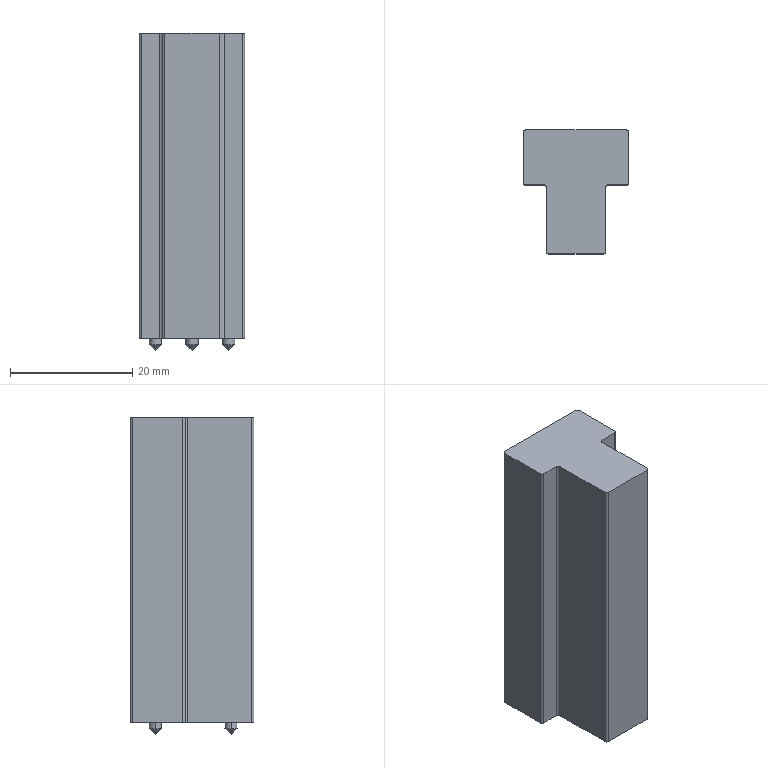Part | Creo | features DATUM PLANE 3, CURVE 2, PROTRUSION 2, CHAMFER 1, COORDINATE SYSTEM 1 | 1 solid | 30 faces | box 17.25 x 20.25 x 52 mm | volume 13253 mm3 | cylinder 14 | plane 10 | cone 6 | commonest cylinder face diameters 0.75 x8 2 x6
STEP:
#1=CARTESIAN_POINT('',(0.,0.,0.));
#2=DIRECTION('',(0.,0.,1.));
#3=DIRECTION('',(1.,0.,0.));
#4=AXIS2_PLACEMENT_3D('',#1,#2,#3);
#5=CARTESIAN_POINT('',(4.87,-9.75,0.));
#6=VERTEX_POINT('',#5);
#7=CARTESIAN_POINT('',(4.87,0.75,0.));
#8=VERTEX_POINT('',#7);
#9=CARTESIAN_POINT('',(4.87,-9.75,0.));
#10=DIRECTION('',(0.,1.,0.));
#11=VECTOR('',#10,10.5);
#12=LINE('',#9,#11);
#13=EDGE_CURVE('',#6,#8,#12,.T.);
#14=ORIENTED_EDGE('',*,*,#13,.T.);
#15=CARTESIAN_POINT('',(5.245,1.125,0.));
#16=VERTEX_POINT('',#15);
#17=CARTESIAN_POINT('',(5.245,0.75,0.));
#18=DIRECTION('',(0.,0.,-1.));
#19=DIRECTION('',(-1.,0.,0.));
#20=AXIS2_PLACEMENT_3D('',#17,#18,#19);
#21=CIRCLE('',#20,0.375);
#22=EDGE_CURVE('',#8,#16,#21,.T.);
#23=ORIENTED_EDGE('',*,*,#22,.T.);
#24=CARTESIAN_POINT('',(8.245,1.125,0.));
#25=VERTEX_POINT('',#24);
#26=CARTESIAN_POINT('',(5.245,1.125,0.));
#27=DIRECTION('',(1.,0.,0.));
#28=VECTOR('',#27,3.);
#29=LINE('',#26,#28);
#30=EDGE_CURVE('',#16,#25,#29,.T.);
#31=ORIENTED_EDGE('',*,*,#30,.T.);
#32=CARTESIAN_POINT('',(8.62,1.5,0.));
#33=VERTEX_POINT('',#32);
#34=CARTESIAN_POINT('',(8.245,1.5,0.));
#35=DIRECTION('',(0.,0.,1.));
#36=DIRECTION('',(0.,-1.,0.));
#37=AXIS2_PLACEMENT_3D('',#34,#35,#36);
#38=CIRCLE('',#37,0.375);
#39=EDGE_CURVE('',#25,#33,#38,.T.);
#40=ORIENTED_EDGE('',*,*,#39,.T.);
#41=CARTESIAN_POINT('',(8.62,9.75,0.));
#42=VERTEX_POINT('',#41);
#43=CARTESIAN_POINT('',(8.62,1.5,0.));
#44=DIRECTION('',(0.,1.,0.));
#45=VECTOR('',#44,8.25);
#46=LINE('',#43,#45);
#47=EDGE_CURVE('',#33,#42,#46,.T.);
#48=ORIENTED_EDGE('',*,*,#47,.T.);
#49=CARTESIAN_POINT('',(8.245,10.125,0.));
#50=VERTEX_POINT('',#49);
#51=CARTESIAN_POINT('',(8.245,9.75,0.));
#52=DIRECTION('',(0.,0.,1.));
#53=DIRECTION('',(1.,0.,0.));
#54=AXIS2_PLACEMENT_3D('',#51,#52,#53);
#55=CIRCLE('',#54,0.375);
#56=EDGE_CURVE('',#42,#50,#55,.T.);
#57=ORIENTED_EDGE('',*,*,#56,.T.);
#58=CARTESIAN_POINT('',(-8.255,10.125,0.));
#59=VERTEX_POINT('',#58);
#60=CARTESIAN_POINT('',(8.245,10.125,0.));
#61=DIRECTION('',(-1.,0.,0.));
#62=VECTOR('',#61,16.5);
#63=LINE('',#60,#62);
#64=EDGE_CURVE('',#50,#59,#63,.T.);
#65=ORIENTED_EDGE('',*,*,#64,.T.);
#66=CARTESIAN_POINT('',(-8.63,9.75,0.));
#67=VERTEX_POINT('',#66);
#68=CARTESIAN_POINT('',(-8.255,9.75,0.));
#69=DIRECTION('',(0.,0.,1.));
#70=DIRECTION('',(0.,1.,0.));
#71=AXIS2_PLACEMENT_3D('',#68,#69,#70);
#72=CIRCLE('',#71,0.375);
#73=EDGE_CURVE('',#59,#67,#72,.T.);
#74=ORIENTED_EDGE('',*,*,#73,.T.);
#75=CARTESIAN_POINT('',(-8.63,1.5,0.));
#76=VERTEX_POINT('',#75);
#77=CARTESIAN_POINT('',(-8.63,9.75,0.));
#78=DIRECTION('',(0.,-1.,0.));
#79=VECTOR('',#78,8.25);
#80=LINE('',#77,#79);
#81=EDGE_CURVE('',#67,#76,#80,.T.);
#82=ORIENTED_EDGE('',*,*,#81,.T.);
#83=CARTESIAN_POINT('',(-8.255,1.125,0.));
#84=VERTEX_POINT('',#83);
#85=CARTESIAN_POINT('',(-8.255,1.5,0.));
#86=DIRECTION('',(0.,0.,1.));
#87=DIRECTION('',(-1.,0.,0.));
#88=AXIS2_PLACEMENT_3D('',#85,#86,#87);
#89=CIRCLE('',#88,0.375);
#90=EDGE_CURVE('',#76,#84,#89,.T.);
#91=ORIENTED_EDGE('',*,*,#90,.T.);
#92=CARTESIAN_POINT('',(-5.255,1.125,0.));
#93=VERTEX_POINT('',#92);
#94=CARTESIAN_POINT('',(-8.255,1.125,0.));
#95=DIRECTION('',(1.,0.,0.));
#96=VECTOR('',#95,3.);
#97=LINE('',#94,#96);
#98=EDGE_CURVE('',#84,#93,#97,.T.);
#99=ORIENTED_EDGE('',*,*,#98,.T.);
#100=CARTESIAN_POINT('',(-4.88,0.75,0.));
#101=VERTEX_POINT('',#100);
#102=CARTESIAN_POINT('',(-5.255,0.75,0.));
#103=DIRECTION('',(0.,0.,-1.));
#104=DIRECTION('',(0.,1.,0.));
#105=AXIS2_PLACEMENT_3D('',#102,#103,#104);
#106=CIRCLE('',#105,0.375);
#107=EDGE_CURVE('',#93,#101,#106,.T.);
#108=ORIENTED_EDGE('',*,*,#107,.T.);
#109=CARTESIAN_POINT('',(-4.88,-9.75,0.));
#110=VERTEX_POINT('',#109);
#111=CARTESIAN_POINT('',(-4.88,0.75,0.));
#112=DIRECTION('',(0.,-1.,0.));
#113=VECTOR('',#112,10.5);
#114=LINE('',#111,#113);
#115=EDGE_CURVE('',#101,#110,#114,.T.);
#116=ORIENTED_EDGE('',*,*,#115,.T.);
#117=CARTESIAN_POINT('',(-4.505,-10.125,0.));
#118=VERTEX_POINT('',#117);
#119=CARTESIAN_POINT('',(-4.505,-9.75,0.));
#120=DIRECTION('',(0.,0.,1.));
#121=DIRECTION('',(-1.,0.,0.));
#122=AXIS2_PLACEMENT_3D('',#119,#120,#121);
#123=CIRCLE('',#122,0.375);
#124=EDGE_CURVE('',#110,#118,#123,.T.);
#125=ORIENTED_EDGE('',*,*,#124,.T.);
#126=CARTESIAN_POINT('',(4.495,-10.125,0.));
#127=VERTEX_POINT('',#126);
#128=CARTESIAN_POINT('',(-4.505,-10.125,0.));
#129=DIRECTION('',(1.,0.,0.));
#130=VECTOR('',#129,9.);
#131=LINE('',#128,#130);
#132=EDGE_CURVE('',#118,#127,#131,.T.);
#133=ORIENTED_EDGE('',*,*,#132,.T.);
#134=CARTESIAN_POINT('',(4.495,-9.75,0.));
#135=DIRECTION('',(0.,0.,1.));
#136=DIRECTION('',(0.,-1.,0.));
#137=AXIS2_PLACEMENT_3D('',#134,#135,#136);
#138=CIRCLE('',#137,0.375);
#139=EDGE_CURVE('',#127,#6,#138,.T.);
#140=ORIENTED_EDGE('',*,*,#139,.T.);
#141=EDGE_LOOP('',(#14,#23,#31,#40,#48,#57,#65,#74,#82,#91,#99,#108,#116,#125,#133,#140));
#142=FACE_OUTER_BOUND('',#141,.F.);
#143=CARTESIAN_POINT('',(7.,6.,0.));
#144=VERTEX_POINT('',#143);
#145=CARTESIAN_POINT('',(5.,6.,0.));
#146=VERTEX_POINT('',#145);
#147=CARTESIAN_POINT('',(6.,6.,0.));
#148=DIRECTION('',(0.,0.,1.));
#149=DIRECTION('',(1.,0.,0.));
#150=AXIS2_PLACEMENT_3D('',#147,#148,#149);
#151=CIRCLE('',#150,1.);
#152=EDGE_CURVE('',#144,#146,#151,.T.);
#153=ORIENTED_EDGE('',*,*,#152,.F.);
#154=CARTESIAN_POINT('',(6.,6.,0.));
#155=DIRECTION('',(0.,0.,1.));
#156=DIRECTION('',(-1.,0.,0.));
#157=AXIS2_PLACEMENT_3D('',#154,#155,#156);
#158=CIRCLE('',#157,1.);
#159=EDGE_CURVE('',#146,#144,#158,.T.);
#160=ORIENTED_EDGE('',*,*,#159,.F.);
#161=EDGE_LOOP('',(#153,#160));
#162=FACE_BOUND('',#161,.F.);
#163=CARTESIAN_POINT('',(-5.,6.,0.));
#164=VERTEX_POINT('',#163);
#165=CARTESIAN_POINT('',(-7.,6.,0.));
#166=VERTEX_POINT('',#165);
#167=CARTESIAN_POINT('',(-6.,6.,0.));
#168=DIRECTION('',(0.,0.,1.));
#169=DIRECTION('',(1.,0.,0.));
#170=AXIS2_PLACEMENT_3D('',#167,#168,#169);
#171=CIRCLE('',#170,1.);
#172=EDGE_CURVE('',#164,#166,#171,.T.);
#173=ORIENTED_EDGE('',*,*,#172,.F.);
#174=CARTESIAN_POINT('',(-6.,6.,0.));
#175=DIRECTION('',(0.,0.,1.));
#176=DIRECTION('',(-1.,0.,0.));
#177=AXIS2_PLACEMENT_3D('',#174,#175,#176);
#178=CIRCLE('',#177,1.);
#179=EDGE_CURVE('',#166,#164,#178,.T.);
#180=ORIENTED_EDGE('',*,*,#179,.F.);
#181=EDGE_LOOP('',(#173,#180));
#182=FACE_BOUND('',#181,.F.);
#183=CARTESIAN_POINT('',(1.,-6.397,0.));
#184=VERTEX_POINT('',#183);
#185=CARTESIAN_POINT('',(-1.,-6.397,0.));
#186=VERTEX_POINT('',#185);
#187=CARTESIAN_POINT('',(0.,-6.397,0.));
#188=DIRECTION('',(0.,0.,1.));
#189=DIRECTION('',(1.,0.,0.));
#190=AXIS2_PLACEMENT_3D('',#187,#188,#189);
#191=CIRCLE('',#190,1.);
#192=EDGE_CURVE('',#184,#186,#191,.T.);
#193=ORIENTED_EDGE('',*,*,#192,.F.);
#194=CARTESIAN_POINT('',(0.,-6.397,0.));
#195=DIRECTION('',(0.,0.,1.));
#196=DIRECTION('',(-1.,0.,0.));
#197=AXIS2_PLACEMENT_3D('',#194,#195,#196);
#198=CIRCLE('',#197,1.);
#199=EDGE_CURVE('',#186,#184,#198,.T.);
#200=ORIENTED_EDGE('',*,*,#199,.F.);
#201=EDGE_LOOP('',(#193,#200));
#202=FACE_BOUND('',#201,.F.);
#203=CARTESIAN_POINT('',(0.,0.,0.));
#204=DIRECTION('',(0.,0.,1.));
#205=DIRECTION('',(1.,0.,0.));
#206=AXIS2_PLACEMENT_3D('',#203,#204,#205);
#207=PLANE('',#206);
#208=ADVANCED_FACE('',(#142,#162,#182,#202),#207,.F.);
#209=ORIENTED_EDGE('',*,*,#13,.F.);
#210=CARTESIAN_POINT('',(4.87,-9.75,50.));
#211=VERTEX_POINT('',#210);
#212=CARTESIAN_POINT('',(4.87,-9.75,0.));
#213=DIRECTION('',(0.,0.,1.));
#214=VECTOR('',#213,50.);
#215=LINE('',#212,#214);
#216=EDGE_CURVE('',#6,#211,#215,.T.);
#217=ORIENTED_EDGE('',*,*,#216,.T.);
#218=CARTESIAN_POINT('',(4.87,0.75,50.));
#219=VERTEX_POINT('',#218);
#220=CARTESIAN_POINT('',(4.87,-9.75,50.));
#221=DIRECTION('',(0.,1.,0.));
#222=VECTOR('',#221,10.5);
#223=LINE('',#220,#222);
#224=EDGE_CURVE('',#211,#219,#223,.T.);
#225=ORIENTED_EDGE('',*,*,#224,.T.);
#226=CARTESIAN_POINT('',(4.87,0.75,0.));
#227=DIRECTION('',(0.,0.,1.));
#228=VECTOR('',#227,50.);
#229=LINE('',#226,#228);
#230=EDGE_CURVE('',#8,#219,#229,.T.);
#231=ORIENTED_EDGE('',*,*,#230,.F.);
#232=EDGE_LOOP('',(#209,#217,#225,#231));
#233=FACE_OUTER_BOUND('',#232,.F.);
#234=CARTESIAN_POINT('',(4.87,-9.75,0.));
#235=DIRECTION('',(1.,0.,0.));
#236=DIRECTION('',(0.,1.,0.));
#237=AXIS2_PLACEMENT_3D('',#234,#235,#236);
#238=PLANE('',#237);
#239=ADVANCED_FACE('',(#233),#238,.T.);
#240=ORIENTED_EDGE('',*,*,#139,.F.);
#241=CARTESIAN_POINT('',(4.495,-10.125,50.));
#242=VERTEX_POINT('',#241);
#243=CARTESIAN_POINT('',(4.495,-10.125,0.));
#244=DIRECTION('',(0.,0.,1.));
#245=VECTOR('',#244,50.);
#246=LINE('',#243,#245);
#247=EDGE_CURVE('',#127,#242,#246,.T.);
#248=ORIENTED_EDGE('',*,*,#247,.T.);
#249=CARTESIAN_POINT('',(4.495,-9.75,50.));
#250=DIRECTION('',(0.,0.,1.));
#251=DIRECTION('',(0.,-1.,0.));
#252=AXIS2_PLACEMENT_3D('',#249,#250,#251);
#253=CIRCLE('',#252,0.375);
#254=EDGE_CURVE('',#242,#211,#253,.T.);
#255=ORIENTED_EDGE('',*,*,#254,.T.);
#256=ORIENTED_EDGE('',*,*,#216,.F.);
#257=EDGE_LOOP('',(#240,#248,#255,#256));
#258=FACE_OUTER_BOUND('',#257,.F.);
#259=CARTESIAN_POINT('',(4.495,-9.75,0.));
#260=DIRECTION('',(0.,0.,1.));
#261=DIRECTION('',(1.,0.,0.));
#262=AXIS2_PLACEMENT_3D('',#259,#260,#261);
#263=CYLINDRICAL_SURFACE('',#262,0.375);
#264=ADVANCED_FACE('',(#258),#263,.T.);
#265=ORIENTED_EDGE('',*,*,#132,.F.);
#266=CARTESIAN_POINT('',(-4.505,-10.125,50.));
#267=VERTEX_POINT('',#266);
#268=CARTESIAN_POINT('',(-4.505,-10.125,0.));
#269=DIRECTION('',(0.,0.,1.));
#270=VECTOR('',#269,50.);
#271=LINE('',#268,#270);
#272=EDGE_CURVE('',#118,#267,#271,.T.);
#273=ORIENTED_EDGE('',*,*,#272,.T.);
#274=CARTESIAN_POINT('',(-4.505,-10.125,50.));
#275=DIRECTION('',(1.,0.,0.));
#276=VECTOR('',#275,9.);
#277=LINE('',#274,#276);
#278=EDGE_CURVE('',#267,#242,#277,.T.);
#279=ORIENTED_EDGE('',*,*,#278,.T.);
#280=ORIENTED_EDGE('',*,*,#247,.F.);
#281=EDGE_LOOP('',(#265,#273,#279,#280));
#282=FACE_OUTER_BOUND('',#281,.F.);
#283=CARTESIAN_POINT('',(-4.505,-10.125,0.));
#284=DIRECTION('',(0.,-1.,0.));
#285=DIRECTION('',(1.,0.,0.));
#286=AXIS2_PLACEMENT_3D('',#283,#284,#285);
#287=PLANE('',#286);
#288=ADVANCED_FACE('',(#282),#287,.T.);
#289=ORIENTED_EDGE('',*,*,#124,.F.);
#290=CARTESIAN_POINT('',(-4.88,-9.75,50.));
#291=VERTEX_POINT('',#290);
#292=CARTESIAN_POINT('',(-4.88,-9.75,0.));
#293=DIRECTION('',(0.,0.,1.));
#294=VECTOR('',#293,50.);
#295=LINE('',#292,#294);
#296=EDGE_CURVE('',#110,#291,#295,.T.);
#297=ORIENTED_EDGE('',*,*,#296,.T.);
#298=CARTESIAN_POINT('',(-4.505,-9.75,50.));
#299=DIRECTION('',(0.,0.,1.));
#300=DIRECTION('',(-1.,0.,0.));
#301=AXIS2_PLACEMENT_3D('',#298,#299,#300);
#302=CIRCLE('',#301,0.375);
#303=EDGE_CURVE('',#291,#267,#302,.T.);
#304=ORIENTED_EDGE('',*,*,#303,.T.);
#305=ORIENTED_EDGE('',*,*,#272,.F.);
#306=EDGE_LOOP('',(#289,#297,#304,#305));
#307=FACE_OUTER_BOUND('',#306,.F.);
#308=CARTESIAN_POINT('',(-4.505,-9.75,0.));
#309=DIRECTION('',(0.,0.,1.));
#310=DIRECTION('',(1.,0.,0.));
#311=AXIS2_PLACEMENT_3D('',#308,#309,#310);
#312=CYLINDRICAL_SURFACE('',#311,0.375);
#313=ADVANCED_FACE('',(#307),#312,.T.);
#314=ORIENTED_EDGE('',*,*,#115,.F.);
#315=CARTESIAN_POINT('',(-4.88,0.75,50.));
#316=VERTEX_POINT('',#315);
#317=CARTESIAN_POINT('',(-4.88,0.75,0.));
#318=DIRECTION('',(0.,0.,1.));
#319=VECTOR('',#318,50.);
#320=LINE('',#317,#319);
#321=EDGE_CURVE('',#101,#316,#320,.T.);
#322=ORIENTED_EDGE('',*,*,#321,.T.);
#323=CARTESIAN_POINT('',(-4.88,0.75,50.));
#324=DIRECTION('',(0.,-1.,0.));
#325=VECTOR('',#324,10.5);
#326=LINE('',#323,#325);
#327=EDGE_CURVE('',#316,#291,#326,.T.);
#328=ORIENTED_EDGE('',*,*,#327,.T.);
#329=ORIENTED_EDGE('',*,*,#296,.F.);
#330=EDGE_LOOP('',(#314,#322,#328,#329));
#331=FACE_OUTER_BOUND('',#330,.F.);
#332=CARTESIAN_POINT('',(-4.88,0.75,0.));
#333=DIRECTION('',(-1.,0.,0.));
#334=DIRECTION('',(0.,-1.,0.));
#335=AXIS2_PLACEMENT_3D('',#332,#333,#334);
#336=PLANE('',#335);
#337=ADVANCED_FACE('',(#331),#336,.T.);
#338=ORIENTED_EDGE('',*,*,#107,.F.);
#339=CARTESIAN_POINT('',(-5.255,1.125,50.));
#340=VERTEX_POINT('',#339);
#341=CARTESIAN_POINT('',(-5.255,1.125,0.));
#342=DIRECTION('',(0.,0.,1.));
#343=VECTOR('',#342,50.);
#344=LINE('',#341,#343);
#345=EDGE_CURVE('',#93,#340,#344,.T.);
#346=ORIENTED_EDGE('',*,*,#345,.T.);
#347=CARTESIAN_POINT('',(-5.255,0.75,50.));
#348=DIRECTION('',(0.,0.,-1.));
#349=DIRECTION('',(0.,1.,0.));
#350=AXIS2_PLACEMENT_3D('',#347,#348,#349);
#351=CIRCLE('',#350,0.375);
#352=EDGE_CURVE('',#340,#316,#351,.T.);
#353=ORIENTED_EDGE('',*,*,#352,.T.);
#354=ORIENTED_EDGE('',*,*,#321,.F.);
#355=EDGE_LOOP('',(#338,#346,#353,#354));
#356=FACE_OUTER_BOUND('',#355,.F.);
#357=CARTESIAN_POINT('',(-5.255,0.75,0.));
#358=DIRECTION('',(0.,0.,1.));
#359=DIRECTION('',(1.,0.,0.));
#360=AXIS2_PLACEMENT_3D('',#357,#358,#359);
#361=CYLINDRICAL_SURFACE('',#360,0.375);
#362=ADVANCED_FACE('',(#356),#361,.F.);
#363=ORIENTED_EDGE('',*,*,#98,.F.);
#364=CARTESIAN_POINT('',(-8.255,1.125,50.));
#365=VERTEX_POINT('',#364);
#366=CARTESIAN_POINT('',(-8.255,1.125,0.));
#367=DIRECTION('',(0.,0.,1.));
#368=VECTOR('',#367,50.);
#369=LINE('',#366,#368);
#370=EDGE_CURVE('',#84,#365,#369,.T.);
#371=ORIENTED_EDGE('',*,*,#370,.T.);
#372=CARTESIAN_POINT('',(-8.255,1.125,50.));
#373=DIRECTION('',(1.,0.,0.));
#374=VECTOR('',#373,3.);
#375=LINE('',#372,#374);
#376=EDGE_CURVE('',#365,#340,#375,.T.);
#377=ORIENTED_EDGE('',*,*,#376,.T.);
#378=ORIENTED_EDGE('',*,*,#345,.F.);
#379=EDGE_LOOP('',(#363,#371,#377,#378));
#380=FACE_OUTER_BOUND('',#379,.F.);
#381=CARTESIAN_POINT('',(-8.255,1.125,0.));
#382=DIRECTION('',(0.,-1.,0.));
#383=DIRECTION('',(1.,0.,0.));
#384=AXIS2_PLACEMENT_3D('',#381,#382,#383);
#385=PLANE('',#384);
#386=ADVANCED_FACE('',(#380),#385,.T.);
#387=ORIENTED_EDGE('',*,*,#90,.F.);
#388=CARTESIAN_POINT('',(-8.63,1.5,50.));
#389=VERTEX_POINT('',#388);
#390=CARTESIAN_POINT('',(-8.63,1.5,0.));
#391=DIRECTION('',(0.,0.,1.));
#392=VECTOR('',#391,50.);
#393=LINE('',#390,#392);
#394=EDGE_CURVE('',#76,#389,#393,.T.);
#395=ORIENTED_EDGE('',*,*,#394,.T.);
#396=CARTESIAN_POINT('',(-8.255,1.5,50.));
#397=DIRECTION('',(0.,0.,1.));
#398=DIRECTION('',(-1.,0.,0.));
#399=AXIS2_PLACEMENT_3D('',#396,#397,#398);
#400=CIRCLE('',#399,0.375);
#401=EDGE_CURVE('',#389,#365,#400,.T.);
#402=ORIENTED_EDGE('',*,*,#401,.T.);
#403=ORIENTED_EDGE('',*,*,#370,.F.);
#404=EDGE_LOOP('',(#387,#395,#402,#403));
#405=FACE_OUTER_BOUND('',#404,.F.);
#406=CARTESIAN_POINT('',(-8.255,1.5,0.));
#407=DIRECTION('',(0.,0.,1.));
#408=DIRECTION('',(1.,0.,0.));
#409=AXIS2_PLACEMENT_3D('',#406,#407,#408);
#410=CYLINDRICAL_SURFACE('',#409,0.375);
#411=ADVANCED_FACE('',(#405),#410,.T.);
#412=ORIENTED_EDGE('',*,*,#81,.F.);
#413=CARTESIAN_POINT('',(-8.63,9.75,50.));
#414=VERTEX_POINT('',#413);
#415=CARTESIAN_POINT('',(-8.63,9.75,0.));
#416=DIRECTION('',(0.,0.,1.));
#417=VECTOR('',#416,50.);
#418=LINE('',#415,#417);
#419=EDGE_CURVE('',#67,#414,#418,.T.);
#420=ORIENTED_EDGE('',*,*,#419,.T.);
#421=CARTESIAN_POINT('',(-8.63,9.75,50.));
#422=DIRECTION('',(0.,-1.,0.));
#423=VECTOR('',#422,8.25);
#424=LINE('',#421,#423);
#425=EDGE_CURVE('',#414,#389,#424,.T.);
#426=ORIENTED_EDGE('',*,*,#425,.T.);
#427=ORIENTED_EDGE('',*,*,#394,.F.);
#428=EDGE_LOOP('',(#412,#420,#426,#427));
#429=FACE_OUTER_BOUND('',#428,.F.);
#430=CARTESIAN_POINT('',(-8.63,9.75,0.));
#431=DIRECTION('',(-1.,0.,0.));
#432=DIRECTION('',(0.,-1.,0.));
#433=AXIS2_PLACEMENT_3D('',#430,#431,#432);
#434=PLANE('',#433);
#435=ADVANCED_FACE('',(#429),#434,.T.);
#436=ORIENTED_EDGE('',*,*,#73,.F.);
#437=CARTESIAN_POINT('',(-8.255,10.125,50.));
#438=VERTEX_POINT('',#437);
#439=CARTESIAN_POINT('',(-8.255,10.125,0.));
#440=DIRECTION('',(0.,0.,1.));
#441=VECTOR('',#440,50.);
#442=LINE('',#439,#441);
#443=EDGE_CURVE('',#59,#438,#442,.T.);
#444=ORIENTED_EDGE('',*,*,#443,.T.);
#445=CARTESIAN_POINT('',(-8.255,9.75,50.));
#446=DIRECTION('',(0.,0.,1.));
#447=DIRECTION('',(0.,1.,0.));
#448=AXIS2_PLACEMENT_3D('',#445,#446,#447);
#449=CIRCLE('',#448,0.375);
#450=EDGE_CURVE('',#438,#414,#449,.T.);
#451=ORIENTED_EDGE('',*,*,#450,.T.);
#452=ORIENTED_EDGE('',*,*,#419,.F.);
#453=EDGE_LOOP('',(#436,#444,#451,#452));
#454=FACE_OUTER_BOUND('',#453,.F.);
#455=CARTESIAN_POINT('',(-8.255,9.75,0.));
#456=DIRECTION('',(0.,0.,1.));
#457=DIRECTION('',(1.,0.,0.));
#458=AXIS2_PLACEMENT_3D('',#455,#456,#457);
#459=CYLINDRICAL_SURFACE('',#458,0.375);
#460=ADVANCED_FACE('',(#454),#459,.T.);
#461=ORIENTED_EDGE('',*,*,#64,.F.);
#462=CARTESIAN_POINT('',(8.245,10.125,50.));
#463=VERTEX_POINT('',#462);
#464=CARTESIAN_POINT('',(8.245,10.125,0.));
#465=DIRECTION('',(0.,0.,1.));
#466=VECTOR('',#465,50.);
#467=LINE('',#464,#466);
#468=EDGE_CURVE('',#50,#463,#467,.T.);
#469=ORIENTED_EDGE('',*,*,#468,.T.);
#470=CARTESIAN_POINT('',(8.245,10.125,50.));
#471=DIRECTION('',(-1.,0.,0.));
#472=VECTOR('',#471,16.5);
#473=LINE('',#470,#472);
#474=EDGE_CURVE('',#463,#438,#473,.T.);
#475=ORIENTED_EDGE('',*,*,#474,.T.);
#476=ORIENTED_EDGE('',*,*,#443,.F.);
#477=EDGE_LOOP('',(#461,#469,#475,#476));
#478=FACE_OUTER_BOUND('',#477,.F.);
#479=CARTESIAN_POINT('',(8.245,10.125,0.));
#480=DIRECTION('',(0.,1.,0.));
#481=DIRECTION('',(-1.,0.,0.));
#482=AXIS2_PLACEMENT_3D('',#479,#480,#481);
#483=PLANE('',#482);
#484=ADVANCED_FACE('',(#478),#483,.T.);
#485=ORIENTED_EDGE('',*,*,#56,.F.);
#486=CARTESIAN_POINT('',(8.62,9.75,50.));
#487=VERTEX_POINT('',#486);
#488=CARTESIAN_POINT('',(8.62,9.75,0.));
#489=DIRECTION('',(0.,0.,1.));
#490=VECTOR('',#489,50.);
#491=LINE('',#488,#490);
#492=EDGE_CURVE('',#42,#487,#491,.T.);
#493=ORIENTED_EDGE('',*,*,#492,.T.);
#494=CARTESIAN_POINT('',(8.245,9.75,50.));
#495=DIRECTION('',(0.,0.,1.));
#496=DIRECTION('',(1.,0.,0.));
#497=AXIS2_PLACEMENT_3D('',#494,#495,#496);
#498=CIRCLE('',#497,0.375);
#499=EDGE_CURVE('',#487,#463,#498,.T.);
#500=ORIENTED_EDGE('',*,*,#499,.T.);
#501=ORIENTED_EDGE('',*,*,#468,.F.);
#502=EDGE_LOOP('',(#485,#493,#500,#501));
#503=FACE_OUTER_BOUND('',#502,.F.);
#504=CARTESIAN_POINT('',(8.245,9.75,0.));
#505=DIRECTION('',(0.,0.,1.));
#506=DIRECTION('',(1.,0.,0.));
#507=AXIS2_PLACEMENT_3D('',#504,#505,#506);
#508=CYLINDRICAL_SURFACE('',#507,0.375);
#509=ADVANCED_FACE('',(#503),#508,.T.);
#510=ORIENTED_EDGE('',*,*,#47,.F.);
#511=CARTESIAN_POINT('',(8.62,1.5,50.));
#512=VERTEX_POINT('',#511);
#513=CARTESIAN_POINT('',(8.62,1.5,0.));
#514=DIRECTION('',(0.,0.,1.));
#515=VECTOR('',#514,50.);
#516=LINE('',#513,#515);
#517=EDGE_CURVE('',#33,#512,#516,.T.);
#518=ORIENTED_EDGE('',*,*,#517,.T.);
#519=CARTESIAN_POINT('',(8.62,1.5,50.));
#520=DIRECTION('',(0.,1.,0.));
#521=VECTOR('',#520,8.25);
#522=LINE('',#519,#521);
#523=EDGE_CURVE('',#512,#487,#522,.T.);
#524=ORIENTED_EDGE('',*,*,#523,.T.);
#525=ORIENTED_EDGE('',*,*,#492,.F.);
#526=EDGE_LOOP('',(#510,#518,#524,#525));
#527=FACE_OUTER_BOUND('',#526,.F.);
#528=CARTESIAN_POINT('',(8.62,1.5,0.));
#529=DIRECTION('',(1.,0.,0.));
#530=DIRECTION('',(0.,1.,0.));
#531=AXIS2_PLACEMENT_3D('',#528,#529,#530);
#532=PLANE('',#531);
#533=ADVANCED_FACE('',(#527),#532,.T.);
#534=ORIENTED_EDGE('',*,*,#39,.F.);
#535=CARTESIAN_POINT('',(8.245,1.125,50.));
#536=VERTEX_POINT('',#535);
#537=CARTESIAN_POINT('',(8.245,1.125,0.));
#538=DIRECTION('',(0.,0.,1.));
#539=VECTOR('',#538,50.);
#540=LINE('',#537,#539);
#541=EDGE_CURVE('',#25,#536,#540,.T.);
#542=ORIENTED_EDGE('',*,*,#541,.T.);
#543=CARTESIAN_POINT('',(8.245,1.5,50.));
#544=DIRECTION('',(0.,0.,1.));
#545=DIRECTION('',(0.,-1.,0.));
#546=AXIS2_PLACEMENT_3D('',#543,#544,#545);
#547=CIRCLE('',#546,0.375);
#548=EDGE_CURVE('',#536,#512,#547,.T.);
#549=ORIENTED_EDGE('',*,*,#548,.T.);
#550=ORIENTED_EDGE('',*,*,#517,.F.);
#551=EDGE_LOOP('',(#534,#542,#549,#550));
#552=FACE_OUTER_BOUND('',#551,.F.);
#553=CARTESIAN_POINT('',(8.245,1.5,0.));
#554=DIRECTION('',(0.,0.,1.));
#555=DIRECTION('',(1.,0.,0.));
#556=AXIS2_PLACEMENT_3D('',#553,#554,#555);
#557=CYLINDRICAL_SURFACE('',#556,0.375);
#558=ADVANCED_FACE('',(#552),#557,.T.);
#559=ORIENTED_EDGE('',*,*,#30,.F.);
#560=CARTESIAN_POINT('',(5.245,1.125,50.));
#561=VERTEX_POINT('',#560);
#562=CARTESIAN_POINT('',(5.245,1.125,0.));
#563=DIRECTION('',(0.,0.,1.));
#564=VECTOR('',#563,50.);
#565=LINE('',#562,#564);
#566=EDGE_CURVE('',#16,#561,#565,.T.);
#567=ORIENTED_EDGE('',*,*,#566,.T.);
#568=CARTESIAN_POINT('',(5.245,1.125,50.));
#569=DIRECTION('',(1.,0.,0.));
#570=VECTOR('',#569,3.);
#571=LINE('',#568,#570);
#572=EDGE_CURVE('',#561,#536,#571,.T.);
#573=ORIENTED_EDGE('',*,*,#572,.T.);
#574=ORIENTED_EDGE('',*,*,#541,.F.);
#575=EDGE_LOOP('',(#559,#567,#573,#574));
#576=FACE_OUTER_BOUND('',#575,.F.);
#577=CARTESIAN_POINT('',(5.245,1.125,0.));
#578=DIRECTION('',(0.,-1.,0.));
#579=DIRECTION('',(1.,0.,0.));
#580=AXIS2_PLACEMENT_3D('',#577,#578,#579);
#581=PLANE('',#580);
#582=ADVANCED_FACE('',(#576),#581,.T.);
#583=ORIENTED_EDGE('',*,*,#22,.F.);
#584=ORIENTED_EDGE('',*,*,#230,.T.);
#585=CARTESIAN_POINT('',(5.245,0.75,50.));
#586=DIRECTION('',(0.,0.,-1.));
#587=DIRECTION('',(-1.,0.,0.));
#588=AXIS2_PLACEMENT_3D('',#585,#586,#587);
#589=CIRCLE('',#588,0.375);
#590=EDGE_CURVE('',#219,#561,#589,.T.);
#591=ORIENTED_EDGE('',*,*,#590,.T.);
#592=ORIENTED_EDGE('',*,*,#566,.F.);
#593=EDGE_LOOP('',(#583,#584,#591,#592));
#594=FACE_OUTER_BOUND('',#593,.F.);
#595=CARTESIAN_POINT('',(5.245,0.75,0.));
#596=DIRECTION('',(0.,0.,1.));
#597=DIRECTION('',(1.,0.,0.));
#598=AXIS2_PLACEMENT_3D('',#595,#596,#597);
#599=CYLINDRICAL_SURFACE('',#598,0.375);
#600=ADVANCED_FACE('',(#594),#599,.F.);
#601=ORIENTED_EDGE('',*,*,#224,.F.);
#602=ORIENTED_EDGE('',*,*,#254,.F.);
#603=ORIENTED_EDGE('',*,*,#278,.F.);
#604=ORIENTED_EDGE('',*,*,#303,.F.);
#605=ORIENTED_EDGE('',*,*,#327,.F.);
#606=ORIENTED_EDGE('',*,*,#352,.F.);
#607=ORIENTED_EDGE('',*,*,#376,.F.);
#608=ORIENTED_EDGE('',*,*,#401,.F.);
#609=ORIENTED_EDGE('',*,*,#425,.F.);
#610=ORIENTED_EDGE('',*,*,#450,.F.);
#611=ORIENTED_EDGE('',*,*,#474,.F.);
#612=ORIENTED_EDGE('',*,*,#499,.F.);
#613=ORIENTED_EDGE('',*,*,#523,.F.);
#614=ORIENTED_EDGE('',*,*,#548,.F.);
#615=ORIENTED_EDGE('',*,*,#572,.F.);
#616=ORIENTED_EDGE('',*,*,#590,.F.);
#617=EDGE_LOOP('',(#601,#602,#603,#604,#605,#606,#607,#608,#609,#610,#611,#612,#613,#614,#615,#616));
#618=FACE_OUTER_BOUND('',#617,.F.);
#619=CARTESIAN_POINT('',(0.,0.,50.));
#620=DIRECTION('',(0.,0.,1.));
#621=DIRECTION('',(1.,0.,0.));
#622=AXIS2_PLACEMENT_3D('',#619,#620,#621);
#623=PLANE('',#622);
#624=ADVANCED_FACE('',(#618),#623,.T.);
#625=CARTESIAN_POINT('',(5.,6.,-1.));
#626=VERTEX_POINT('',#625);
#627=CARTESIAN_POINT('',(7.,6.,-1.));
#628=VERTEX_POINT('',#627);
#629=CARTESIAN_POINT('',(6.,6.,-1.));
#630=DIRECTION('',(0.,0.,-1.));
#631=DIRECTION('',(-1.,0.,0.));
#632=AXIS2_PLACEMENT_3D('',#629,#630,#631);
#633=CIRCLE('',#632,1.);
#634=EDGE_CURVE('',#626,#628,#633,.T.);
#635=ORIENTED_EDGE('',*,*,#634,.T.);
#636=CARTESIAN_POINT('',(7.,6.,-1.));
#637=DIRECTION('',(0.000000003,0.000000017,1.));
#638=VECTOR('',#637,1.);
#639=LINE('',#636,#638);
#640=EDGE_CURVE('',#628,#144,#639,.T.);
#641=ORIENTED_EDGE('',*,*,#640,.T.);
#642=ORIENTED_EDGE('',*,*,#152,.T.);
#643=CARTESIAN_POINT('',(5.,6.,-1.));
#644=DIRECTION('',(-0.000000003,-0.000000017,1.));
#645=VECTOR('',#644,1.);
#646=LINE('',#643,#645);
#647=EDGE_CURVE('',#626,#146,#646,.T.);
#648=ORIENTED_EDGE('',*,*,#647,.F.);
#649=EDGE_LOOP('',(#635,#641,#642,#648));
#650=FACE_OUTER_BOUND('',#649,.F.);
#651=CARTESIAN_POINT('',(6.,6.,50.));
#652=DIRECTION('',(0.,0.,1.));
#653=DIRECTION('',(1.,0.,0.));
#654=AXIS2_PLACEMENT_3D('',#651,#652,#653);
#655=CYLINDRICAL_SURFACE('',#654,1.);
#656=ADVANCED_FACE('',(#650),#655,.T.);
#657=ORIENTED_EDGE('',*,*,#634,.F.);
#658=CARTESIAN_POINT('',(6.,6.,-2.));
#659=VERTEX_POINT('',#658);
#660=CARTESIAN_POINT('',(6.,6.,-2.));
#661=DIRECTION('',(-0.7071,0.000000012,0.7071));
#662=VECTOR('',#661,1.414);
#663=LINE('',#660,#662);
#664=EDGE_CURVE('',#659,#626,#663,.T.);
#665=ORIENTED_EDGE('',*,*,#664,.F.);
#666=CARTESIAN_POINT('',(6.,6.,-2.));
#667=DIRECTION('',(0.7071,-0.000000012,0.7071));
#668=VECTOR('',#667,1.414);
#669=LINE('',#666,#668);
#670=EDGE_CURVE('',#659,#628,#669,.T.);
#671=ORIENTED_EDGE('',*,*,#670,.T.);
#672=EDGE_LOOP('',(#657,#665,#671));
#673=FACE_OUTER_BOUND('',#672,.F.);
#674=CARTESIAN_POINT('',(6.,6.,-1.475));
#675=DIRECTION('',(0.,0.,1.));
#676=DIRECTION('',(0.,-1.,0.));
#677=AXIS2_PLACEMENT_3D('',#674,#675,#676);
#678=CONICAL_SURFACE('',#677,0.5248,45.);
#679=ADVANCED_FACE('',(#673),#678,.T.);
#680=CARTESIAN_POINT('',(6.,6.,-1.));
#681=DIRECTION('',(0.,0.,-1.));
#682=DIRECTION('',(1.,0.,0.));
#683=AXIS2_PLACEMENT_3D('',#680,#681,#682);
#684=CIRCLE('',#683,1.);
#685=EDGE_CURVE('',#628,#626,#684,.T.);
#686=ORIENTED_EDGE('',*,*,#685,.F.);
#687=ORIENTED_EDGE('',*,*,#670,.F.);
#688=ORIENTED_EDGE('',*,*,#664,.T.);
#689=EDGE_LOOP('',(#686,#687,#688));
#690=FACE_OUTER_BOUND('',#689,.F.);
#691=CARTESIAN_POINT('',(6.,6.,-1.475));
#692=DIRECTION('',(0.,0.,1.));
#693=DIRECTION('',(0.,-1.,0.));
#694=AXIS2_PLACEMENT_3D('',#691,#692,#693);
#695=CONICAL_SURFACE('',#694,0.5248,45.);
#696=ADVANCED_FACE('',(#690),#695,.T.);
#697=ORIENTED_EDGE('',*,*,#685,.T.);
#698=ORIENTED_EDGE('',*,*,#647,.T.);
#699=ORIENTED_EDGE('',*,*,#159,.T.);
#700=ORIENTED_EDGE('',*,*,#640,.F.);
#701=EDGE_LOOP('',(#697,#698,#699,#700));
#702=FACE_OUTER_BOUND('',#701,.F.);
#703=CARTESIAN_POINT('',(6.,6.,50.));
#704=DIRECTION('',(0.,0.,1.));
#705=DIRECTION('',(1.,0.,0.));
#706=AXIS2_PLACEMENT_3D('',#703,#704,#705);
#707=CYLINDRICAL_SURFACE('',#706,1.);
#708=ADVANCED_FACE('',(#702),#707,.T.);
#709=CARTESIAN_POINT('',(-7.,6.,-1.));
#710=VERTEX_POINT('',#709);
#711=CARTESIAN_POINT('',(-5.,6.,-1.));
#712=VERTEX_POINT('',#711);
#713=CARTESIAN_POINT('',(-6.,6.,-1.));
#714=DIRECTION('',(0.,0.,-1.));
#715=DIRECTION('',(-1.,0.,0.));
#716=AXIS2_PLACEMENT_3D('',#713,#714,#715);
#717=CIRCLE('',#716,1.);
#718=EDGE_CURVE('',#710,#712,#717,.T.);
#719=ORIENTED_EDGE('',*,*,#718,.T.);
#720=CARTESIAN_POINT('',(-5.,6.,-1.));
#721=DIRECTION('',(0.000000003,0.000000017,1.));
#722=VECTOR('',#721,1.);
#723=LINE('',#720,#722);
#724=EDGE_CURVE('',#712,#164,#723,.T.);
#725=ORIENTED_EDGE('',*,*,#724,.T.);
#726=ORIENTED_EDGE('',*,*,#172,.T.);
#727=CARTESIAN_POINT('',(-7.,6.,-1.));
#728=DIRECTION('',(-0.000000003,-0.000000017,1.));
#729=VECTOR('',#728,1.);
#730=LINE('',#727,#729);
#731=EDGE_CURVE('',#710,#166,#730,.T.);
#732=ORIENTED_EDGE('',*,*,#731,.F.);
#733=EDGE_LOOP('',(#719,#725,#726,#732));
#734=FACE_OUTER_BOUND('',#733,.F.);
#735=CARTESIAN_POINT('',(-6.,6.,50.));
#736=DIRECTION('',(0.,0.,1.));
#737=DIRECTION('',(1.,0.,0.));
#738=AXIS2_PLACEMENT_3D('',#735,#736,#737);
#739=CYLINDRICAL_SURFACE('',#738,1.);
#740=ADVANCED_FACE('',(#734),#739,.T.);
#741=ORIENTED_EDGE('',*,*,#718,.F.);
#742=CARTESIAN_POINT('',(-6.,6.,-2.));
#743=VERTEX_POINT('',#742);
#744=CARTESIAN_POINT('',(-6.,6.,-2.));
#745=DIRECTION('',(-0.7071,0.000000012,0.7071));
#746=VECTOR('',#745,1.414);
#747=LINE('',#744,#746);
#748=EDGE_CURVE('',#743,#710,#747,.T.);
#749=ORIENTED_EDGE('',*,*,#748,.F.);
#750=CARTESIAN_POINT('',(-6.,6.,-2.));
#751=DIRECTION('',(0.7071,-0.000000012,0.7071));
#752=VECTOR('',#751,1.414);
#753=LINE('',#750,#752);
#754=EDGE_CURVE('',#743,#712,#753,.T.);
#755=ORIENTED_EDGE('',*,*,#754,.T.);
#756=EDGE_LOOP('',(#741,#749,#755));
#757=FACE_OUTER_BOUND('',#756,.F.);
#758=CARTESIAN_POINT('',(-6.,6.,-1.475));
#759=DIRECTION('',(0.,0.,1.));
#760=DIRECTION('',(0.,-1.,0.));
#761=AXIS2_PLACEMENT_3D('',#758,#759,#760);
#762=CONICAL_SURFACE('',#761,0.5248,45.);
#763=ADVANCED_FACE('',(#757),#762,.T.);
#764=CARTESIAN_POINT('',(-6.,6.,-1.));
#765=DIRECTION('',(0.,0.,-1.));
#766=DIRECTION('',(1.,0.,0.));
#767=AXIS2_PLACEMENT_3D('',#764,#765,#766);
#768=CIRCLE('',#767,1.);
#769=EDGE_CURVE('',#712,#710,#768,.T.);
#770=ORIENTED_EDGE('',*,*,#769,.F.);
#771=ORIENTED_EDGE('',*,*,#754,.F.);
#772=ORIENTED_EDGE('',*,*,#748,.T.);
#773=EDGE_LOOP('',(#770,#771,#772));
#774=FACE_OUTER_BOUND('',#773,.F.);
#775=CARTESIAN_POINT('',(-6.,6.,-1.475));
#776=DIRECTION('',(0.,0.,1.));
#777=DIRECTION('',(0.,-1.,0.));
#778=AXIS2_PLACEMENT_3D('',#775,#776,#777);
#779=CONICAL_SURFACE('',#778,0.5248,45.);
#780=ADVANCED_FACE('',(#774),#779,.T.);
#781=ORIENTED_EDGE('',*,*,#769,.T.);
#782=ORIENTED_EDGE('',*,*,#731,.T.);
#783=ORIENTED_EDGE('',*,*,#179,.T.);
#784=ORIENTED_EDGE('',*,*,#724,.F.);
#785=EDGE_LOOP('',(#781,#782,#783,#784));
#786=FACE_OUTER_BOUND('',#785,.F.);
#787=CARTESIAN_POINT('',(-6.,6.,50.));
#788=DIRECTION('',(0.,0.,1.));
#789=DIRECTION('',(1.,0.,0.));
#790=AXIS2_PLACEMENT_3D('',#787,#788,#789);
#791=CYLINDRICAL_SURFACE('',#790,1.);
#792=ADVANCED_FACE('',(#786),#791,.T.);
#793=CARTESIAN_POINT('',(-1.,-6.397,-1.));
#794=VERTEX_POINT('',#793);
#795=CARTESIAN_POINT('',(1.,-6.397,-1.));
#796=VERTEX_POINT('',#795);
#797=CARTESIAN_POINT('',(0.,-6.397,-1.));
#798=DIRECTION('',(0.,0.,-1.));
#799=DIRECTION('',(-1.,0.,0.));
#800=AXIS2_PLACEMENT_3D('',#797,#798,#799);
#801=CIRCLE('',#800,1.);
#802=EDGE_CURVE('',#794,#796,#801,.T.);
#803=ORIENTED_EDGE('',*,*,#802,.T.);
#804=CARTESIAN_POINT('',(1.,-6.397,-1.));
#805=DIRECTION('',(0.000000003,0.000000017,1.));
#806=VECTOR('',#805,1.);
#807=LINE('',#804,#806);
#808=EDGE_CURVE('',#796,#184,#807,.T.);
#809=ORIENTED_EDGE('',*,*,#808,.T.);
#810=ORIENTED_EDGE('',*,*,#192,.T.);
#811=CARTESIAN_POINT('',(-1.,-6.397,-1.));
#812=DIRECTION('',(-0.000000003,-0.000000017,1.));
#813=VECTOR('',#812,1.);
#814=LINE('',#811,#813);
#815=EDGE_CURVE('',#794,#186,#814,.T.);
#816=ORIENTED_EDGE('',*,*,#815,.F.);
#817=EDGE_LOOP('',(#803,#809,#810,#816));
#818=FACE_OUTER_BOUND('',#817,.F.);
#819=CARTESIAN_POINT('',(0.,-6.397,50.));
#820=DIRECTION('',(0.,0.,1.));
#821=DIRECTION('',(1.,0.,0.));
#822=AXIS2_PLACEMENT_3D('',#819,#820,#821);
#823=CYLINDRICAL_SURFACE('',#822,1.);
#824=ADVANCED_FACE('',(#818),#823,.T.);
#825=ORIENTED_EDGE('',*,*,#802,.F.);
#826=CARTESIAN_POINT('',(0.,-6.397,-2.));
#827=VERTEX_POINT('',#826);
#828=CARTESIAN_POINT('',(0.,-6.397,-2.));
#829=DIRECTION('',(-0.7071,0.000000012,0.7071));
#830=VECTOR('',#829,1.414);
#831=LINE('',#828,#830);
#832=EDGE_CURVE('',#827,#794,#831,.T.);
#833=ORIENTED_EDGE('',*,*,#832,.F.);
#834=CARTESIAN_POINT('',(0.,-6.397,-2.));
#835=DIRECTION('',(0.7071,-0.000000012,0.7071));
#836=VECTOR('',#835,1.414);
#837=LINE('',#834,#836);
#838=EDGE_CURVE('',#827,#796,#837,.T.);
#839=ORIENTED_EDGE('',*,*,#838,.T.);
#840=EDGE_LOOP('',(#825,#833,#839));
#841=FACE_OUTER_BOUND('',#840,.F.);
#842=CARTESIAN_POINT('',(0.,-6.397,-1.475));
#843=DIRECTION('',(0.,0.,1.));
#844=DIRECTION('',(0.,-1.,0.));
#845=AXIS2_PLACEMENT_3D('',#842,#843,#844);
#846=CONICAL_SURFACE('',#845,0.5248,45.);
#847=ADVANCED_FACE('',(#841),#846,.T.);
#848=CARTESIAN_POINT('',(0.,-6.397,-1.));
#849=DIRECTION('',(0.,0.,-1.));
#850=DIRECTION('',(1.,0.,0.));
#851=AXIS2_PLACEMENT_3D('',#848,#849,#850);
#852=CIRCLE('',#851,1.);
#853=EDGE_CURVE('',#796,#794,#852,.T.);
#854=ORIENTED_EDGE('',*,*,#853,.F.);
#855=ORIENTED_EDGE('',*,*,#838,.F.);
#856=ORIENTED_EDGE('',*,*,#832,.T.);
#857=EDGE_LOOP('',(#854,#855,#856));
#858=FACE_OUTER_BOUND('',#857,.F.);
#859=CARTESIAN_POINT('',(0.,-6.397,-1.475));
#860=DIRECTION('',(0.,0.,1.));
#861=DIRECTION('',(0.,-1.,0.));
#862=AXIS2_PLACEMENT_3D('',#859,#860,#861);
#863=CONICAL_SURFACE('',#862,0.5248,45.);
#864=ADVANCED_FACE('',(#858),#863,.T.);
#865=ORIENTED_EDGE('',*,*,#853,.T.);
#866=ORIENTED_EDGE('',*,*,#815,.T.);
#867=ORIENTED_EDGE('',*,*,#199,.T.);
#868=ORIENTED_EDGE('',*,*,#808,.F.);
#869=EDGE_LOOP('',(#865,#866,#867,#868));
#870=FACE_OUTER_BOUND('',#869,.F.);
#871=CARTESIAN_POINT('',(0.,-6.397,50.));
#872=DIRECTION('',(0.,0.,1.));
#873=DIRECTION('',(1.,0.,0.));
#874=AXIS2_PLACEMENT_3D('',#871,#872,#873);
#875=CYLINDRICAL_SURFACE('',#874,1.);
#876=ADVANCED_FACE('',(#870),#875,.T.);
#877=CLOSED_SHELL('',(#208,#239,#264,#288,#313,#337,#362,#386,#411,#435,#460,#484,#509,#533,#558,#582,#600,#624,#656,#679,#696,#708,#740,#763,#780,#792,#824,#847,#864,#876));
#878=MANIFOLD_SOLID_BREP('',#877);
#879=(LENGTH_UNIT()NAMED_UNIT(*)SI_UNIT(.MILLI.,.METRE.));
#880=UNCERTAINTY_MEASURE_WITH_UNIT(LENGTH_MEASURE(0.005841),#879,'','');
#881=(NAMED_UNIT(*)PLANE_ANGLE_UNIT()SI_UNIT($,.RADIAN.));
#882=PLANE_ANGLE_MEASURE_WITH_UNIT(PLANE_ANGLE_MEASURE(0.01745),#881);
#883=(CONVERSION_BASED_UNIT('DEGREE',#882)NAMED_UNIT(*)PLANE_ANGLE_UNIT());
#884=(NAMED_UNIT(*)SI_UNIT($,.STERADIAN.)SOLID_ANGLE_UNIT());
#885=(GEOMETRIC_REPRESENTATION_CONTEXT(3)GLOBAL_UNCERTAINTY_ASSIGNED_CONTEXT((#880))GLOBAL_UNIT_ASSIGNED_CONTEXT((#879,#883,#884))REPRESENTATION_CONTEXT('',''));
#886=ADVANCED_BREP_SHAPE_REPRESENTATION('',(#4,#878),#885);